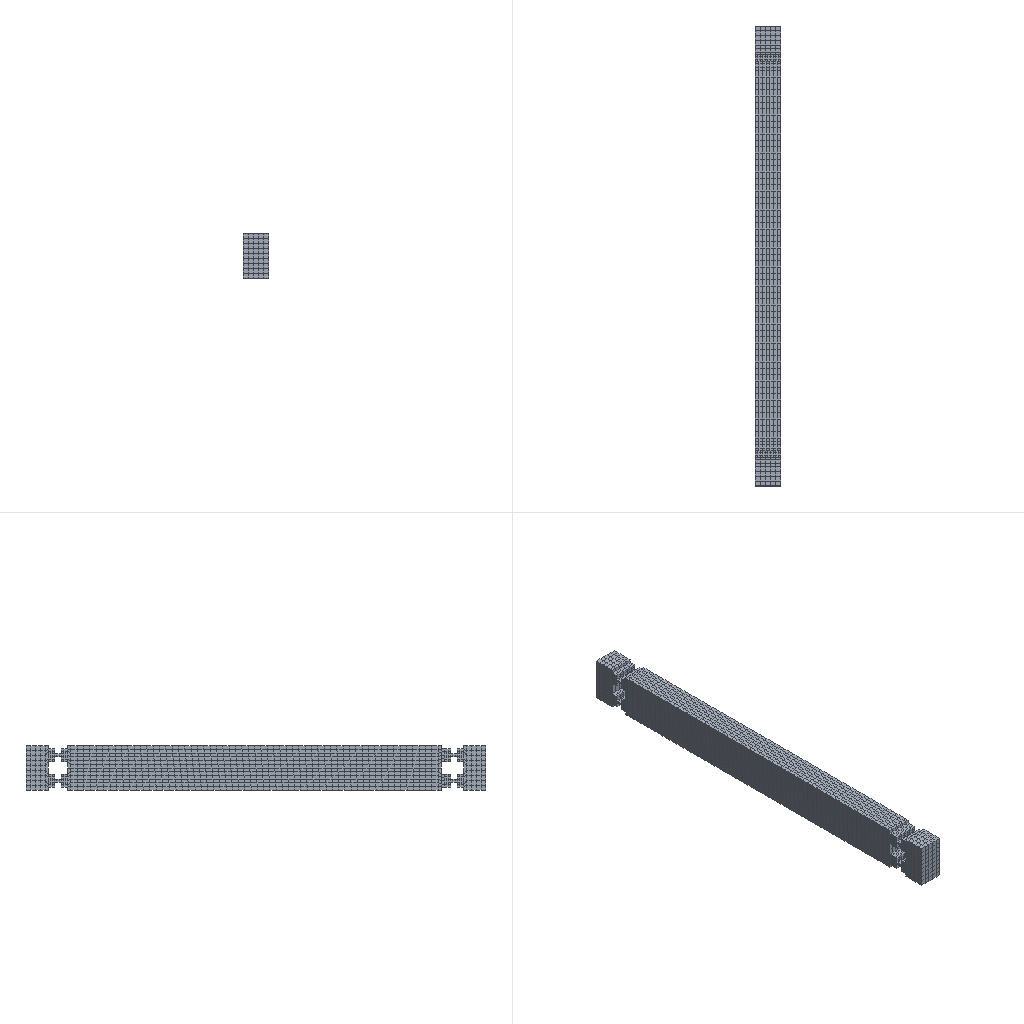Simulation study | abaqus
Set-up summary:
category,name,step,type,value,unit,region
solver,abaqus
solver,version,,,Abaqus/Standard 2020
units,not stated in the deck,,not stated
analysis,deck,,static,static
load_step,Step-1,Step-1,static
load_step,requested,,,1
mesh,nodes,,,10087
mesh,elements,,,7424
element_type,T3D2,,truss,910
element_type,C3D8R,,solid,6514
load,load commands in deck,,count,2
bc,support commands in deck,,count,7
material,CON,,in results
material,STEEEL,,in results
material,STEEL,,in results
check,setup vs results,,match,"per instance, exact: element labels, types and connectivity; labels of the nodes the elements use; coordinates of those nodes at SINGLE_PRECISION in 3 of 9 instance(s)"
Abaqus input file, long lists of numbers shortened:
*Heading
** Job name: Job-1 Model name: Model-1
** Generated by: Abaqus/CAE 2020
*Preprint, echo=NO, model=NO, history=NO, contact=NO
**
** PARTS
**
*Part, name=merge
*Node
      1,          25.,       -2875.,          25.
      2,          25.,       -2875.,         275.
** (840 more lines like these left out)
*Element, type=T3D2
 1,  2, 53
 2, 53, 54
** (888 more lines like these left out)
*Nset, nset=Set-3
   1,   2,   3,   4,   5,   6,   7,   8,   9,  10,  11,  12,  13,  14,  15,  16
  17,  18,  19,  20,  21,  22,  23,  24,  25,  26,  27,  28,  29,  30,  31,  32
** (24 more lines like these left out)
*Elset, elset=Set-3
   1,   2,   3,   4,   5,   6,   7,   8,   9,  10,  11,  12,  13,  14,  15,  16
 137, 138, 139, 140, 141, 142, 143, 144, 145, 146, 157, 158, 159, 160, 161, 162
** (24 more lines like these left out)
*Nset, nset=Set-4
   1,   2,   3,   4,   5,   6,   7,   8,   9,  10,  11,  12,  13,  14,  15,  16
  17,  18,  19,  20,  21,  22,  23,  24,  25,  26,  27,  28,  29,  30,  31,  32
** (28 more lines like these left out)
*Elset, elset=Set-4
  17,  18,  19,  20,  21,  22,  23,  24,  25,  26,  27,  28,  29,  30,  31,  32
  33,  34,  35,  36,  37,  38,  39,  40,  41,  42,  43,  44,  45,  46,  47,  48
** (28 more lines like these left out)
** Section: Section-10
*Solid Section, elset=Set-3, material=steel
78.5,
** Section: Section-12
*Solid Section, elset=Set-4, material=steel
113.04,
*End Part
**
*Part, name=prt0001
*Node
      1,           0.,          55.,         325.
      2,           0.,          55.,         305.
** (6806 more lines like these left out)
*Element, type=C3D8R
1, 156, 163, 162, 145,   1,   2,   3,   4
2, 155, 164, 161, 146, 156, 163, 162, 145
** (5262 more lines like these left out)
*Nset, nset=Set-3, generate
    1,  6808,     1
*Elset, elset=Set-3, generate
    1,  5264,     1
*Nset, nset=Set-4
   96,   97,   99,  100,  129,  130,  131,  132,  133,  134,  135,  136,  137,  138,  139,  140
  453,  454,  455,  456,  457,  458,  459,  460,  461,  462,  463,  465,  466,  467,  468,  469
** (382 more lines like these left out)
*Elset, elset=Set-4, generate
  309,  5180,     1
*Nset, nset=Set-5
    1,    2,    3,    4,    5,    6,    7,    8,    9,   10,   11,   12,   13,   14,   15,   16
   17,   18,   19,   20,   21,   22,   23,   24,   25,   26,   27,   28,   29,   30,   31,   32
** (53 more lines like these left out)
*Elset, elset=Set-5
    1,    2,    3,    4,    5,    6,    7,    8,    9,   10,   11,   12,   13,   14,   15,   16
   17,   18,   19,   20,   21,   22,   23,   24,   25,   26,   27,   28,   29,   30,   31,   32
** (23 more lines like these left out)
** Section: steel
*Solid Section, elset=Set-5, material=steel
,
** Section: con
*Solid Section, elset=Set-4, material=con
,
*End Part
**
*Part, name=prt0002
*Node
      1,   1506.715,           0.,   196.729
      2,   1506.715,           0.,   176.729
** (502 more lines like these left out)
*Element, type=C3D8R
 1,  78,  87, 257,  71,   1,   2,  69,   5
 2,  87,  83,  82, 257,   2,   3,   4,  69
** (283 more lines like these left out)
*Nset, nset=Set-1
  58,  59,  61,  62,  65,  66,  67,  68, 189, 190, 191, 192, 193, 194, 195, 196
 197, 198, 199, 200, 201, 202, 203, 204, 213, 214, 215, 216, 217, 218, 219, 220
** (17 more lines like these left out)
*Elset, elset=Set-1, generate
 106,  285,    1
*Nset, nset=Set-2
   1,   2,   3,   4,   5,   6,   7,   8,   9,  10,  11,  12,  13,  14,  15,  16
  17,  18,  19,  20,  21,  22,  23,  24,  25,  26,  27,  28,  29,  30,  31,  32
** (15 more lines like these left out)
*Elset, elset=Set-2, generate
   1,  105,    1
** Section: steel
*Solid Section, elset=Set-2, material=steel
,
** Section: con
*Solid Section, elset=Set-1, material=con
,
*End Part
**
*Part, name=wanqu
*Node
      1,       -1790.,           0.,           0.
      2,           0.,         -50.,           0.
** (19 more lines like these left out)
*Element, type=T3D2
 1,  1,  4
 2,  4,  5
** (18 more lines like these left out)
*Nset, nset=Set-2, generate
  1,  21,   1
*Elset, elset=Set-2, generate
  1,  20,   1
** Section: steel-high
*Solid Section, elset=Set-2, material=steeel
300.,
*End Part
**
*Part, name=xiao
*Node
      1,           0.,         -60.,           0.
      2,           0.,           0.,           0.
** (350 more lines like these left out)
*Element, type=C3D8R
  1,  12,  11,  29,  28,  44,  43,  61,  60
  2,  13,  29,  31,  14,  45,  61,  63,  46
** (168 more lines like these left out)
*Nset, nset=Set-1, generate
   1,  352,    1
*Elset, elset=Set-1, generate
   1,  170,    1
** Section: steel
*Solid Section, elset=Set-1, material=steel
,
*End Part
**
**
** ASSEMBLY
**
*Assembly, name=Assembly
**
*Instance, name=prt0001-1, part=prt0001
*End Instance
**
*Instance, name=prt0002-1, part=prt0002
        200., -4551.715,   128.271
        200., -4551.715,   128.271,         200., -4551.715, 129.271, 90.
*End Instance
**
*Instance, name=xiao-1, part=xiao
          0.,    25.005,         105.
          0.,    25.005,         105., 0.5774, 25.582, 105.577,         120.
*End Instance
**
*Instance, name=xiao-1-lin-1-2, part=xiao
          0.,    25.005,         305.
          0.,    25.005,         305., 0.5774, 25.582, 305.577,         120.
*End Instance
**
*Instance, name=xiao-1-lin-2-1, part=xiao
          0., -3074.995,         105.
          0., -3074.995,         105., 0.5774, -3074.418, 105.577,         120.
*End Instance
**
*Instance, name=xiao-1-lin-2-2, part=xiao
          0., -3074.995,         305.
          0., -3074.995,         305., 0.5774, -3074.418, 305.577,         120.
*End Instance
**
*Instance, name=merge-1, part=merge
          0.,           0.,          25.
*End Instance
**
*Instance, name=wanqu-1, part=wanqu
        100.,       -1460.,         175.
        100.,       -1460.,         175., 99.423, -1460.577, 175.577,         120.
*End Instance
**
*Instance, name=prt0002-2, part=prt0002
          0.,  1651.72,   128.271
          0.,  1651.72,   128.271,           0.,  1651.72, 127.271, 90.
*End Instance
**
*Node
      1,         100.,      -1437.5,           0.
*Nset, nset=Set-1, instance=wanqu-1, generate
  1,  21,   1
*Elset, elset=Set-1, instance=wanqu-1, generate
  1,  20,   1
*Nset, nset=Set-2, instance=wanqu-1, generate
  1,  21,   1
*Elset, elset=Set-2, instance=wanqu-1, generate
  1,  20,   1
*Nset, nset=Set-5, instance=prt0002-1
  58,  61,  65,  67, 217, 218, 219, 220, 221, 222, 223, 235, 236, 237, 253, 254
 255, 256, 365, 366, 367, 368, 369, 370, 371, 372, 373, 374, 375, 376
*Nset, nset=Set-5, instance=prt0002-2
  58,  61,  65,  67, 217, 218, 219, 220, 221, 222, 223, 235, 236, 237, 253, 254
 255, 256, 365, 366, 367, 368, 369, 370, 371, 372, 373, 374, 375, 376
*Elset, elset=Set-5, instance=prt0002-1, generate
 114,  285,    9
*Elset, elset=Set-5, instance=prt0002-2, generate
 114,  285,    9
*Nset, nset=Set-7
 1,
*Nset, nset=m_Set-3, instance=merge-1, generate
   1,  842,    1
*Elset, elset=m_Set-3, instance=merge-1, generate
   1,  890,    1
*Nset, nset=m_Set-6
 1,
*Nset, nset=s_Set-3, instance=prt0001-1
   96,   97,   99,  100,  129,  130,  131,  132,  133,  134,  135,  136,  137,  138,  139,  140
  453,  454,  455,  456,  457,  458,  459,  460,  461,  462,  463,  465,  466,  467,  468,  469
** (382 more lines like these left out)
*Elset, elset=s_Set-3, instance=prt0001-1, generate
  309,  5180,     1
*Elset, elset=_m_Surf-1_END1, internal, instance=wanqu-1
 11,
*Surface, type=ELEMENT, name=m_Surf-1
_m_Surf-1_END1, END1
*Elset, elset=_m_Surf-3_END1, internal, instance=wanqu-1
 1,
*Surface, type=ELEMENT, name=m_Surf-3
_m_Surf-3_END1, END1
*Elset, elset=_s_Surf-1_S6, internal, instance=prt0002-2, generate
  65,  101,    9
*Surface, type=ELEMENT, name=s_Surf-1
_s_Surf-1_S6, S6
*Elset, elset=_s_Surf-3_S6, internal, instance=prt0002-1, generate
  65,  101,    9
*Surface, type=ELEMENT, name=s_Surf-3
_s_Surf-3_S6, S6
*Elset, elset=_s_Surf-5_S4, internal, instance=prt0001-1
  524,  536,  548,  788,  800,  812, 1220, 1232, 1244, 1484, 1496, 1508, 1916, 1928, 1940, 2180
 2192, 2204, 2612, 2624, 2636, 2876, 2888, 2900, 3308, 3320, 3332, 3572, 3584, 3596, 4004, 4016
** (1 more lines like these left out)
*Surface, type=ELEMENT, name=s_Surf-5
_s_Surf-5_S4, S4
** Constraint: Constraint-1
*Embedded Element, host elset=s_Set-3
m_Set-3
** Constraint: Constraint-2
*Tie, name=Constraint-2, adjust=yes
s_Surf-1, m_Surf-1
** Constraint: Constraint-3
*Tie, name=Constraint-3, adjust=yes
s_Surf-3, m_Surf-3
** Constraint: Constraint-4
*Coupling, constraint name=Constraint-4, ref node=m_Set-6, surface=s_Surf-5
*Kinematic
*End Assembly
*Amplitude, name=Amp-1
             0.,              0.,              1.,              1.
**
** MATERIALS
**
*Material, name=con
*Density
 2.2e-09,
*Elastic
29791., 0.2
*Concrete Damaged Plasticity
30.,    0.1,   1.16, 0.6667,   0.05
*Concrete Compression Hardening
 15.4,      0.
 16.9,  0.0002
 19.6, 0.00048
 20.1, 0.00079
  20., 0.00095
 19.6,  0.0011
 19.1, 0.00127
 18.6, 0.00143
 17.9,  0.0016
 17.2, 0.00177
 16.6, 0.00194
 15.9, 0.00211
 15.3, 0.00228
 14.7, 0.00245
 14.1, 0.00261
 13.5, 0.00278
  13., 0.00294
 12.5,  0.0031
  12., 0.00327
 11.6, 0.00343
 11.2, 0.00359
 10.8, 0.00375
 10.4, 0.00391
 10.1, 0.00406
*Concrete Tension Stiffening
 2.06,      0.
 1.92,   2e-05
 1.72,   4e-05
 1.53,   6e-05
 1.37,   8e-05
 1.24,  0.0001
 1.13, 0.00011
 1.04, 0.00013
 0.97, 0.00015
  0.9, 0.00016
 0.85, 0.00018
*Concrete Compression Damage
     0.,      0.
 0.0841,   9e-05
 0.0933,  0.0001
 0.1091, 0.00013
 0.1418,  0.0002
 0.2407, 0.00048
  0.322, 0.00079
 0.3557, 0.00095
 0.3886,  0.0011
 0.4201, 0.00127
 0.4499, 0.00143
 0.4778,  0.0016
 0.5039, 0.00177
 0.5282, 0.00194
 0.5506, 0.00211
 0.5715, 0.00228
 0.5908, 0.00245
 0.6086, 0.00261
 0.6252, 0.00278
 0.6406, 0.00294
 0.6549,  0.0031
 0.6682, 0.00327
 0.6806, 0.00343
 0.6922, 0.00359
  0.703, 0.00375
 0.7131, 0.00391
 0.7227, 0.00406
   0.74, 0.00438
 0.7554, 0.00469
 0.7691,   0.005
 0.7815, 0.00531
 0.7926, 0.00561
 0.8026, 0.00592
 0.8118, 0.00622
 0.8202, 0.00653
 0.8278, 0.00683
 0.8349, 0.00713
*Concrete Tension Damage
      0.,      0.
 0.1181,   2e-05
 0.2281,   4e-05
 0.3187,   6e-05
 0.3919,   8e-05
 0.4512,  0.0001
 0.5, 0.00011
  0.5407, 0.00013
 0.575, 0.00015
 0.6043, 0.00016
 0.6297, 0.00018
 0.7177, 0.00025
 0.7702, 0.00033
 0.8053,  0.0004
 0.8304, 0.00047
 0.8494, 0.00054
  0.8643, 0.00061
 0.8763, 0.00068
 0.8862, 0.00075
*Material, name=steeel
*Density
 7.8e-09,
*Elastic
210000., 0.3
*Expansion
 1.5e-05,
*Plastic
600.,0.
*Material, name=steel
*Density
 7.8e-09,
*Elastic
210000., 0.3
*Plastic
300.,0.
**
** INTERACTION PROPERTIES
**
*Surface Interaction, name=IntProp-1
1.,
*Friction, slip tolerance=0.005
 0.3,
*Surface Behavior, pressure-overclosure=HARD
**
** BOUNDARY CONDITIONS
**
** Name: BC-1 Type: 对称/反对称/完全固定
*Boundary
Set-5, ENCASTRE
**
** PREDEFINED FIELDS
**
** Name: Predefined Field-1   Type: Temperature
*Initial Conditions, type=TEMPERATURE
Set-1, 300.
**
** INTERACTIONS
**
** Interaction: Int-1
*Contact
*Contact Inclusions, ALL EXTERIOR
*Contact Property Assignment
 ,  , IntProp-1
** ----------------------------------------------------------------
**
** STEP: Step-1
**
*Step, name=Step-1, nlgeom=YES, inc=1000
*Static, stabilize=0.0002, allsdtol=0.05, continue=NO
0.01, 1., 1e-05, 1.
**
** BOUNDARY CONDITIONS
**
** Name: BC-2 Type: 位移/转角
*Boundary, amplitude=Amp-1
Set-7, 1, 1
Set-7, 2, 2
Set-7, 3, 3, 40.
Set-7, 4, 4
Set-7, 5, 5
Set-7, 6, 6
**
** PREDEFINED FIELDS
**
** Name: Predefined Field-2   Type: Temperature
*Temperature
Set-2, 100.
**
** OUTPUT REQUESTS
**
*Restart, write, frequency=0
**
** FIELD OUTPUT: F-Output-1
**
*Output, field
*Node Output
CF, NT, RF, U, V
*Element Output, directions=YES
DAMAGEC, DAMAGET, E, LE, MISES, MISESMAX, PE, PEEQ, PEMAG, S, SDEG, SSAVG, TEMP, TSHR
*Contact Output
CDISP, CSTRESS
**
** HISTORY OUTPUT: H-Output-1
**
*Output, history, variable=PRESELECT
*End Step
Results summary:
result,step,,completed,increments=60 time=1.0/1.0
result,analysis,,,static
result,last_loadstep,,,1
result,primary field,,,U
result,reaction total,,FX,0.001592,model units
result,reaction total,,FY,-13.097,model units
result,reaction total,,FZ,2970.438,model units